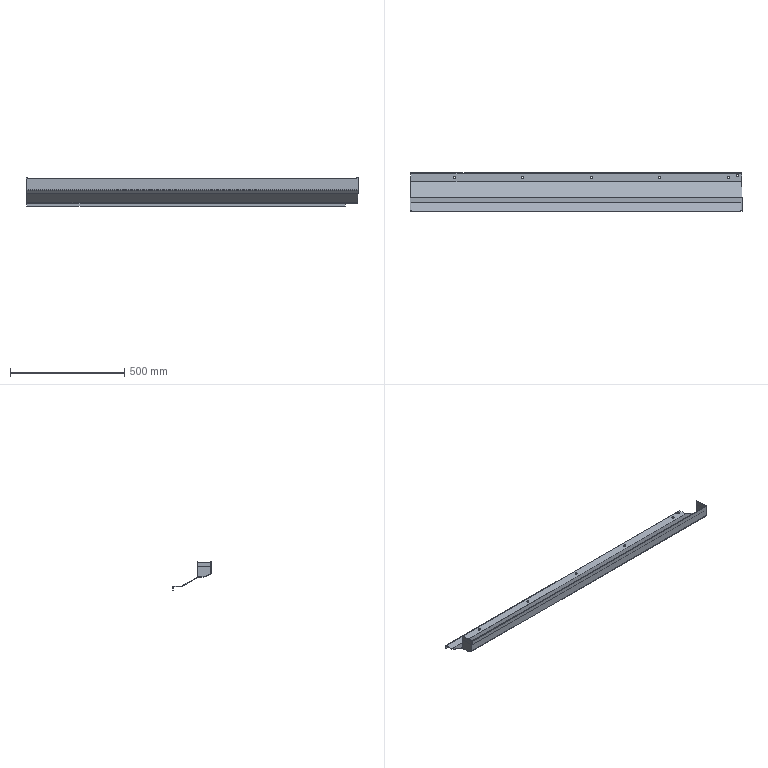Part | NX | features solid 2 | 1 solid | 103 faces | box 1454 x 168 x 123.002 mm | volume 786537 mm3 | plane 65 | cylinder 38 | commonest cylinder face diameters 10 x12 4 x7 8 x7 1 x6 0.004 x3 4.004 x3